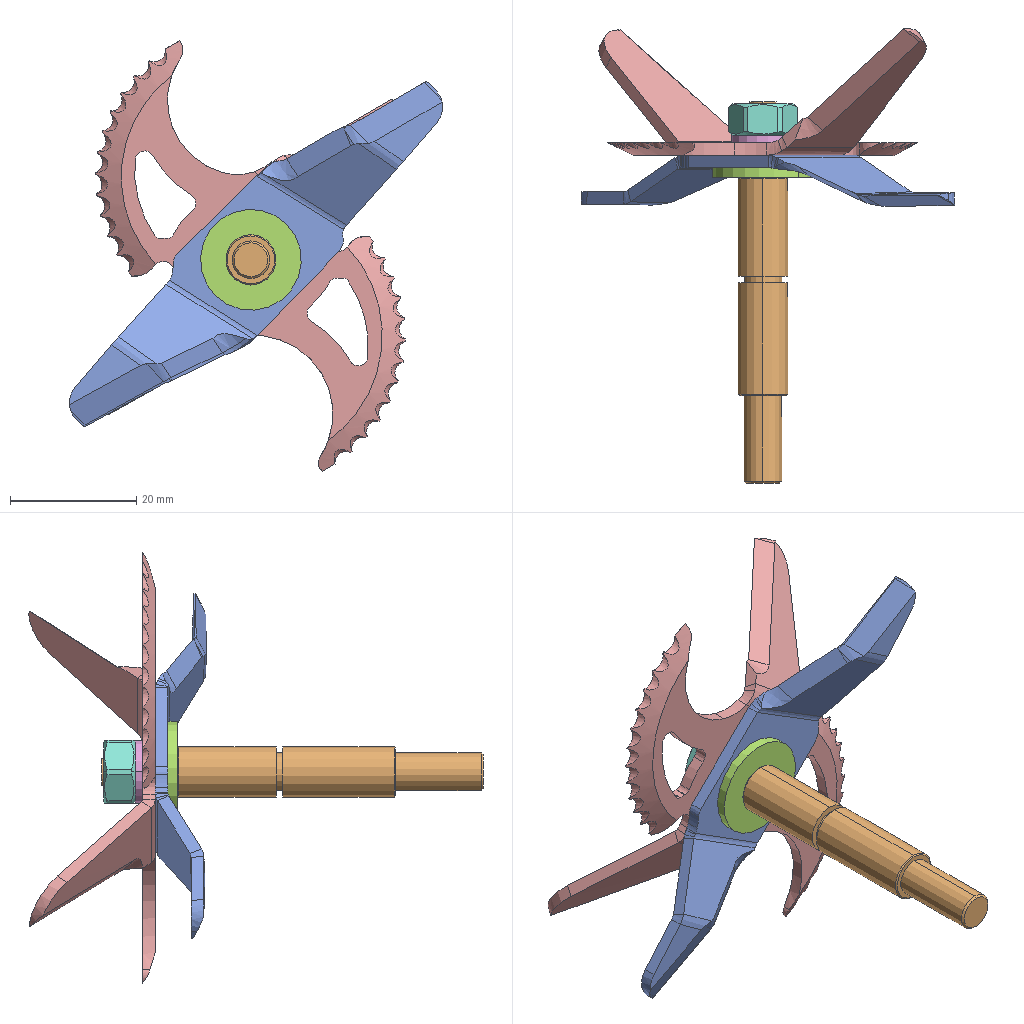Assembly | SolidWorks | 6 different items | 6 placed | box 59 x 72 x 68 mm
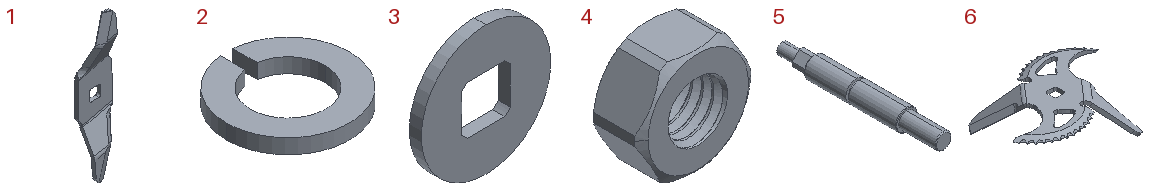Parts list (item | quantity | size | volume | features):
1 | x1 | 18.18 x 8.128 x 77.268 mm | 1719 mm3 | features 3DProfileFeature 4, SM3dBend 4, SweepCut 2, Cut 1, Fillet 1, FlatPattern 1, SMBaseFlange 1, SheetMetal 1
2 | x1 | 10 x 9.975 x 1.2 mm | 56.832 mm3 | features Extrusion 1
3 | x1 | 16 x 1.5 x 16 mm | 248.819 mm3 | features Extrusion 1
4 | x1 | 11.05 x 5 x 10 mm | 308.187 mm3 | features BaseBody 1, Chamfer 1
5 | x1 | 8 x 60.5 x 8 mm | 2374 mm3 | features ICE 3, Chamfer 2, Revolution 1
6 | x1 | 68.715 x 52.833 x 20.056 mm | 2844 mm3 | features 3DProfileFeature 12, SweepCut 5, ICE 4, CirPattern 2, SM3dBend 2, Cut 1, FlatPattern 1, SMBaseFlange 1, SheetMetal 1
Mates (type | each side: item.copy, entity, surface, feature):
Concentric | 3.1 face cylinder Boss-Extrude1 | 5.1 face cylinder Revolve1
Parallel | 3.1 face plane Boss-Extrude1 | 5.1 face plane Boss-Extrude2
Coincident | 3.1 face plane Boss-Extrude1 | 5.1 face plane Revolve1
Parallel | 1.1 face plane Cut-Extrude1 | 5.1 face plane Boss-Extrude2
Coincident | 1.1 face plane Base-Flange1 | 3.1 face plane Boss-Extrude1
Coincident | 1.1 face plane Cut-Extrude1 | 5.1 face plane Boss-Extrude2
Lock | 1.1 select_type:0 | 5.1 select_type:0
Coincident | 5.1 plane | assembly plane | 3 times
Coincident | 6.1 face plane Base-Flange1 | 1.1 face plane Base-Flange1
Concentric | 2.1 face cylinder Boss-Extrude1 | 5.1 face cylinder Boss-Extrude3
Coincident | 6.1 face plane Base-Flange1 | 2.1 face plane Boss-Extrude1
Concentric | 4.1 edge | 5.1 face cylinder Boss-Extrude3
Coincident | 2.1 face plane Boss-Extrude1 | 4.1 face plane Imported3
Lock | 6.1 select_type:0 | 5.1 select_type:0